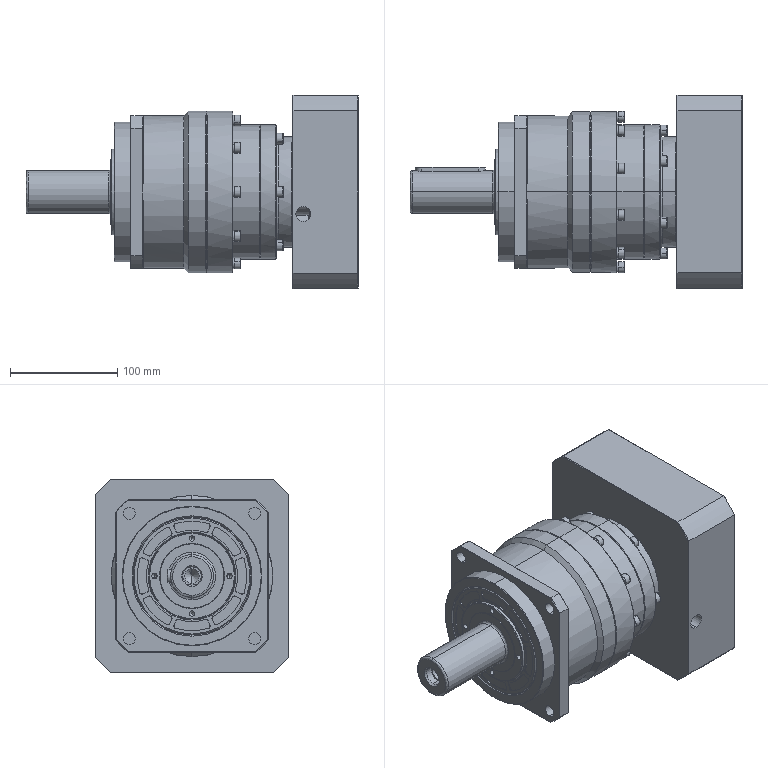Part | SolidWorks | features BaseBody 51 | 51 solids | 1355 faces | box 309 x 180 x 180 mm | volume 4002627 mm3 | plane 594 | cylinder 483 | cone 228 | spline 50 | commonest cylinder face diameters 6.68 x66 9.88 x66 4 x55 6 x44 10 x44 5 x32